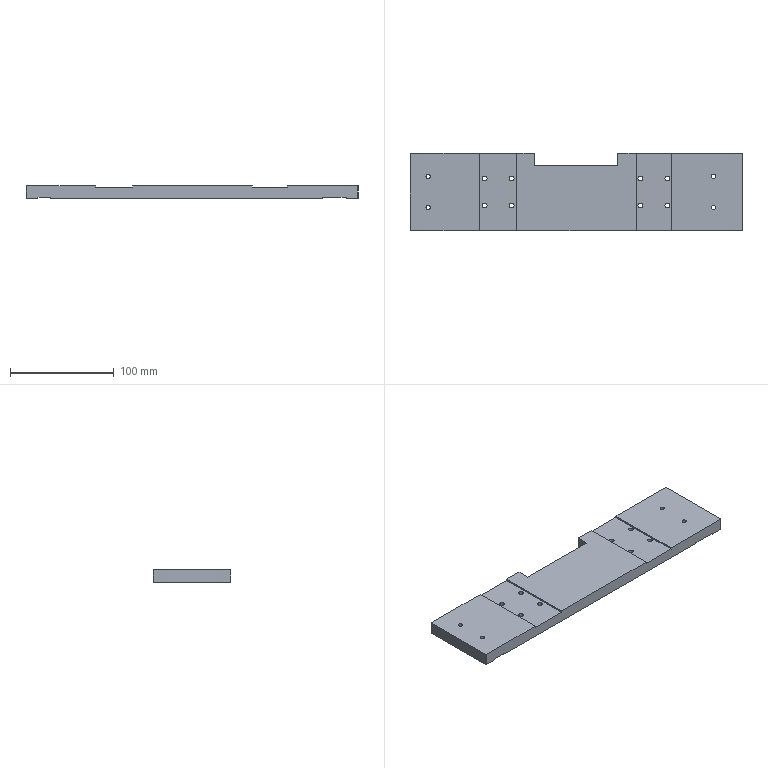Part | STEP file | PN_0088 transport section connecting plate A | 1 solid | 90 faces | box 320 x 75 x 12 mm | volume 262093 mm3 | cylinder 46 | plane 38 | cone 6 | commonest cylinder face diameters 4.5 x16 8 x16 4.2 x14